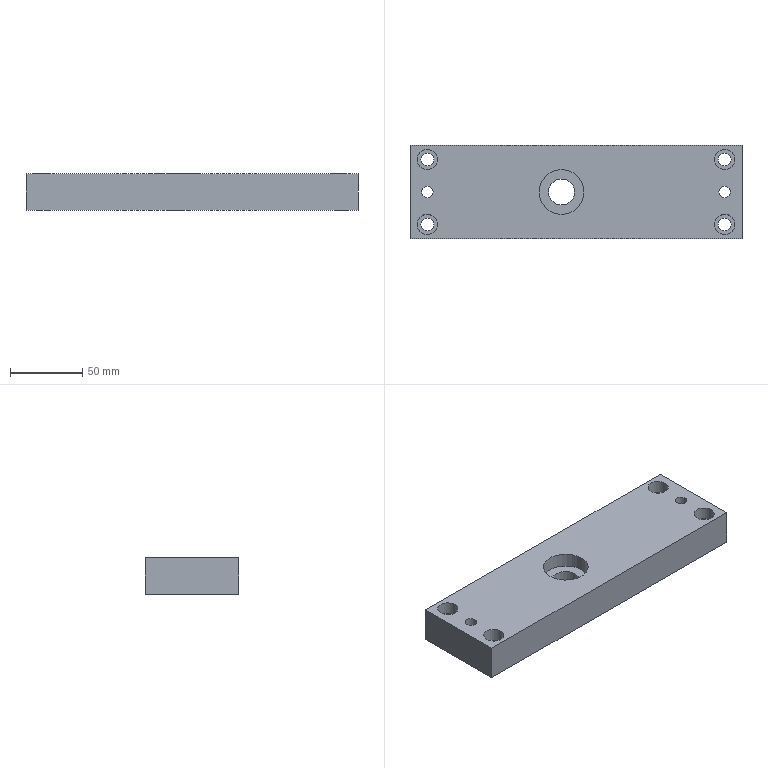Part | STEP file | HYDRAULIC-CYLINDER-BASE2_id482_x_t | 1 solid | 23 faces | box 230 x 65 x 25 mm | volume 350259 mm3 | cylinder 12 | plane 11 | commonest cylinder face diameters 9 x4 14 x4 8 x2 18 x1 31 x1
STEP:
#1=CARTESIAN_POINT('',(90.,-72.5,291.));
#2=VERTEX_POINT('',#1);
#3=CARTESIAN_POINT('',(83.,-72.5,291.));
#4=DIRECTION('',(0.,0.,1.));
#5=DIRECTION('',(1.,0.,0.));
#6=AXIS2_PLACEMENT_3D('',#3,#4,#5);
#7=CIRCLE('',#6,7.);
#8=EDGE_CURVE('',#2,#2,#7,.T.);
#9=ORIENTED_EDGE('',*,*,#8,.F.);
#10=EDGE_LOOP('',(#9));
#11=FACE_BOUND('',#10,.T.);
#12=CARTESIAN_POINT('',(90.,-72.5,300.));
#13=VERTEX_POINT('',#12);
#14=CARTESIAN_POINT('',(83.,-72.5,300.));
#15=DIRECTION('',(0.,0.,-1.));
#16=DIRECTION('',(1.,0.,0.));
#17=AXIS2_PLACEMENT_3D('',#14,#15,#16);
#18=CIRCLE('',#17,7.);
#19=EDGE_CURVE('',#13,#13,#18,.T.);
#20=ORIENTED_EDGE('',*,*,#19,.F.);
#21=EDGE_LOOP('',(#20));
#22=FACE_BOUND('',#21,.T.);
#23=CARTESIAN_POINT('',(83.,-72.5,300.));
#24=DIRECTION('',(0.,0.,1.));
#25=DIRECTION('',(1.,0.,0.));
#26=AXIS2_PLACEMENT_3D('',#23,#24,#25);
#27=CYLINDRICAL_SURFACE('',#26,7.);
#28=ADVANCED_FACE('',(#11,#22),#27,.F.);
#29=CARTESIAN_POINT('',(90.,-27.5,291.));
#30=VERTEX_POINT('',#29);
#31=CARTESIAN_POINT('',(83.,-27.5,291.));
#32=DIRECTION('',(0.,0.,1.));
#33=DIRECTION('',(1.,0.,0.));
#34=AXIS2_PLACEMENT_3D('',#31,#32,#33);
#35=CIRCLE('',#34,7.);
#36=EDGE_CURVE('',#30,#30,#35,.T.);
#37=ORIENTED_EDGE('',*,*,#36,.F.);
#38=EDGE_LOOP('',(#37));
#39=FACE_BOUND('',#38,.T.);
#40=CARTESIAN_POINT('',(90.,-27.5,300.));
#41=VERTEX_POINT('',#40);
#42=CARTESIAN_POINT('',(83.,-27.5,300.));
#43=DIRECTION('',(0.,0.,-1.));
#44=DIRECTION('',(1.,0.,0.));
#45=AXIS2_PLACEMENT_3D('',#42,#43,#44);
#46=CIRCLE('',#45,7.);
#47=EDGE_CURVE('',#41,#41,#46,.T.);
#48=ORIENTED_EDGE('',*,*,#47,.F.);
#49=EDGE_LOOP('',(#48));
#50=FACE_BOUND('',#49,.T.);
#51=CARTESIAN_POINT('',(83.,-27.5,300.));
#52=DIRECTION('',(0.,0.,1.));
#53=DIRECTION('',(1.,0.,0.));
#54=AXIS2_PLACEMENT_3D('',#51,#52,#53);
#55=CYLINDRICAL_SURFACE('',#54,7.);
#56=ADVANCED_FACE('',(#39,#50),#55,.F.);
#57=CARTESIAN_POINT('',(-116.,-27.5,291.));
#58=VERTEX_POINT('',#57);
#59=CARTESIAN_POINT('',(-123.,-27.5,291.));
#60=DIRECTION('',(0.,0.,1.));
#61=DIRECTION('',(1.,0.,0.));
#62=AXIS2_PLACEMENT_3D('',#59,#60,#61);
#63=CIRCLE('',#62,7.);
#64=EDGE_CURVE('',#58,#58,#63,.T.);
#65=ORIENTED_EDGE('',*,*,#64,.F.);
#66=EDGE_LOOP('',(#65));
#67=FACE_BOUND('',#66,.T.);
#68=CARTESIAN_POINT('',(-116.,-27.5,300.));
#69=VERTEX_POINT('',#68);
#70=CARTESIAN_POINT('',(-123.,-27.5,300.));
#71=DIRECTION('',(0.,0.,-1.));
#72=DIRECTION('',(1.,0.,0.));
#73=AXIS2_PLACEMENT_3D('',#70,#71,#72);
#74=CIRCLE('',#73,7.);
#75=EDGE_CURVE('',#69,#69,#74,.T.);
#76=ORIENTED_EDGE('',*,*,#75,.F.);
#77=EDGE_LOOP('',(#76));
#78=FACE_BOUND('',#77,.T.);
#79=CARTESIAN_POINT('',(-123.,-27.5,300.));
#80=DIRECTION('',(0.,0.,1.));
#81=DIRECTION('',(1.,0.,0.));
#82=AXIS2_PLACEMENT_3D('',#79,#80,#81);
#83=CYLINDRICAL_SURFACE('',#82,7.);
#84=ADVANCED_FACE('',(#67,#78),#83,.F.);
#85=CARTESIAN_POINT('',(-116.,-72.5,291.));
#86=VERTEX_POINT('',#85);
#87=CARTESIAN_POINT('',(-123.,-72.5,291.));
#88=DIRECTION('',(0.,0.,1.));
#89=DIRECTION('',(1.,0.,0.));
#90=AXIS2_PLACEMENT_3D('',#87,#88,#89);
#91=CIRCLE('',#90,7.);
#92=EDGE_CURVE('',#86,#86,#91,.T.);
#93=ORIENTED_EDGE('',*,*,#92,.F.);
#94=EDGE_LOOP('',(#93));
#95=FACE_BOUND('',#94,.T.);
#96=CARTESIAN_POINT('',(-116.,-72.5,300.));
#97=VERTEX_POINT('',#96);
#98=CARTESIAN_POINT('',(-123.,-72.5,300.));
#99=DIRECTION('',(0.,0.,-1.));
#100=DIRECTION('',(1.,0.,0.));
#101=AXIS2_PLACEMENT_3D('',#98,#99,#100);
#102=CIRCLE('',#101,7.);
#103=EDGE_CURVE('',#97,#97,#102,.T.);
#104=ORIENTED_EDGE('',*,*,#103,.F.);
#105=EDGE_LOOP('',(#104));
#106=FACE_BOUND('',#105,.T.);
#107=CARTESIAN_POINT('',(-123.,-72.5,300.));
#108=DIRECTION('',(0.,0.,1.));
#109=DIRECTION('',(1.,0.,0.));
#110=AXIS2_PLACEMENT_3D('',#107,#108,#109);
#111=CYLINDRICAL_SURFACE('',#110,7.);
#112=ADVANCED_FACE('',(#95,#106),#111,.F.);
#113=CARTESIAN_POINT('',(-14.5,-50.,290.));
#114=VERTEX_POINT('',#113);
#115=CARTESIAN_POINT('',(-30.,-50.,290.));
#116=DIRECTION('',(0.,0.,1.));
#117=DIRECTION('',(1.,0.,0.));
#118=AXIS2_PLACEMENT_3D('',#115,#116,#117);
#119=CIRCLE('',#118,15.5);
#120=EDGE_CURVE('',#114,#114,#119,.T.);
#121=ORIENTED_EDGE('',*,*,#120,.F.);
#122=EDGE_LOOP('',(#121));
#123=FACE_BOUND('',#122,.T.);
#124=CARTESIAN_POINT('',(-14.5,-50.,300.));
#125=VERTEX_POINT('',#124);
#126=CARTESIAN_POINT('',(-30.,-50.,300.));
#127=DIRECTION('',(0.,0.,-1.));
#128=DIRECTION('',(1.,0.,0.));
#129=AXIS2_PLACEMENT_3D('',#126,#127,#128);
#130=CIRCLE('',#129,15.5);
#131=EDGE_CURVE('',#125,#125,#130,.T.);
#132=ORIENTED_EDGE('',*,*,#131,.F.);
#133=EDGE_LOOP('',(#132));
#134=FACE_BOUND('',#133,.T.);
#135=CARTESIAN_POINT('',(-30.,-50.,300.));
#136=DIRECTION('',(0.,0.,1.));
#137=DIRECTION('',(1.,0.,0.));
#138=AXIS2_PLACEMENT_3D('',#135,#136,#137);
#139=CYLINDRICAL_SURFACE('',#138,15.5);
#140=ADVANCED_FACE('',(#123,#134),#139,.F.);
#141=CARTESIAN_POINT('',(87.5,-27.5,291.));
#142=VERTEX_POINT('',#141);
#143=CARTESIAN_POINT('',(83.,-27.5,291.));
#144=DIRECTION('',(0.,0.,-1.));
#145=DIRECTION('',(1.,0.,0.));
#146=AXIS2_PLACEMENT_3D('',#143,#144,#145);
#147=CIRCLE('',#146,4.5);
#148=EDGE_CURVE('',#142,#142,#147,.T.);
#149=ORIENTED_EDGE('',*,*,#148,.T.);
#150=EDGE_LOOP('',(#149));
#151=FACE_BOUND('',#150,.T.);
#152=ORIENTED_EDGE('',*,*,#36,.T.);
#153=EDGE_LOOP('',(#152));
#154=FACE_BOUND('',#153,.T.);
#155=CARTESIAN_POINT('',(50.126,-0.5,291.));
#156=DIRECTION('',(0.,0.,1.));
#157=DIRECTION('',(1.,0.,0.));
#158=AXIS2_PLACEMENT_3D('',#155,#156,#157);
#159=PLANE('',#158);
#160=ADVANCED_FACE('',(#151,#154),#159,.T.);
#161=CARTESIAN_POINT('',(87.5,-72.5,291.));
#162=VERTEX_POINT('',#161);
#163=CARTESIAN_POINT('',(83.,-72.5,291.));
#164=DIRECTION('',(0.,0.,-1.));
#165=DIRECTION('',(1.,0.,0.));
#166=AXIS2_PLACEMENT_3D('',#163,#164,#165);
#167=CIRCLE('',#166,4.5);
#168=EDGE_CURVE('',#162,#162,#167,.T.);
#169=ORIENTED_EDGE('',*,*,#168,.T.);
#170=EDGE_LOOP('',(#169));
#171=FACE_BOUND('',#170,.T.);
#172=ORIENTED_EDGE('',*,*,#8,.T.);
#173=EDGE_LOOP('',(#172));
#174=FACE_BOUND('',#173,.T.);
#175=CARTESIAN_POINT('',(50.126,-0.5,291.));
#176=DIRECTION('',(0.,0.,1.));
#177=DIRECTION('',(1.,0.,0.));
#178=AXIS2_PLACEMENT_3D('',#175,#176,#177);
#179=PLANE('',#178);
#180=ADVANCED_FACE('',(#171,#174),#179,.T.);
#181=CARTESIAN_POINT('',(-118.5,-27.5,291.));
#182=VERTEX_POINT('',#181);
#183=CARTESIAN_POINT('',(-123.,-27.5,291.));
#184=DIRECTION('',(0.,0.,-1.));
#185=DIRECTION('',(1.,0.,0.));
#186=AXIS2_PLACEMENT_3D('',#183,#184,#185);
#187=CIRCLE('',#186,4.5);
#188=EDGE_CURVE('',#182,#182,#187,.T.);
#189=ORIENTED_EDGE('',*,*,#188,.T.);
#190=EDGE_LOOP('',(#189));
#191=FACE_BOUND('',#190,.T.);
#192=ORIENTED_EDGE('',*,*,#64,.T.);
#193=EDGE_LOOP('',(#192));
#194=FACE_BOUND('',#193,.T.);
#195=CARTESIAN_POINT('',(50.126,-0.5,291.));
#196=DIRECTION('',(0.,0.,1.));
#197=DIRECTION('',(1.,0.,0.));
#198=AXIS2_PLACEMENT_3D('',#195,#196,#197);
#199=PLANE('',#198);
#200=ADVANCED_FACE('',(#191,#194),#199,.T.);
#201=ORIENTED_EDGE('',*,*,#131,.T.);
#202=EDGE_LOOP('',(#201));
#203=FACE_BOUND('',#202,.T.);
#204=ORIENTED_EDGE('',*,*,#75,.T.);
#205=EDGE_LOOP('',(#204));
#206=FACE_BOUND('',#205,.T.);
#207=ORIENTED_EDGE('',*,*,#103,.T.);
#208=EDGE_LOOP('',(#207));
#209=FACE_BOUND('',#208,.T.);
#210=ORIENTED_EDGE('',*,*,#47,.T.);
#211=EDGE_LOOP('',(#210));
#212=FACE_BOUND('',#211,.T.);
#213=ORIENTED_EDGE('',*,*,#19,.T.);
#214=EDGE_LOOP('',(#213));
#215=FACE_BOUND('',#214,.T.);
#216=CARTESIAN_POINT('',(-119.,-50.,300.));
#217=VERTEX_POINT('',#216);
#218=CARTESIAN_POINT('',(-123.,-50.,300.));
#219=DIRECTION('',(0.,0.,-1.));
#220=DIRECTION('',(1.,0.,0.));
#221=AXIS2_PLACEMENT_3D('',#218,#219,#220);
#222=CIRCLE('',#221,4.);
#223=EDGE_CURVE('',#217,#217,#222,.T.);
#224=ORIENTED_EDGE('',*,*,#223,.T.);
#225=EDGE_LOOP('',(#224));
#226=FACE_BOUND('',#225,.T.);
#227=CARTESIAN_POINT('',(87.,-50.,300.));
#228=VERTEX_POINT('',#227);
#229=CARTESIAN_POINT('',(83.,-50.,300.));
#230=DIRECTION('',(0.,0.,-1.));
#231=DIRECTION('',(1.,0.,0.));
#232=AXIS2_PLACEMENT_3D('',#229,#230,#231);
#233=CIRCLE('',#232,4.);
#234=EDGE_CURVE('',#228,#228,#233,.T.);
#235=ORIENTED_EDGE('',*,*,#234,.T.);
#236=EDGE_LOOP('',(#235));
#237=FACE_BOUND('',#236,.T.);
#238=CARTESIAN_POINT('',(95.,-17.5,300.));
#239=VERTEX_POINT('',#238);
#240=CARTESIAN_POINT('',(95.,-82.5,300.));
#241=VERTEX_POINT('',#240);
#242=CARTESIAN_POINT('',(95.,-82.5,300.));
#243=DIRECTION('',(0.,-1.,0.));
#244=VECTOR('',#243,1.);
#245=LINE('',#242,#244);
#246=EDGE_CURVE('',#239,#241,#245,.T.);
#247=ORIENTED_EDGE('',*,*,#246,.F.);
#248=CARTESIAN_POINT('',(-135.,-17.5,300.));
#249=VERTEX_POINT('',#248);
#250=CARTESIAN_POINT('',(95.,-17.5,300.));
#251=DIRECTION('',(1.,0.,0.));
#252=VECTOR('',#251,1.);
#253=LINE('',#250,#252);
#254=EDGE_CURVE('',#249,#239,#253,.T.);
#255=ORIENTED_EDGE('',*,*,#254,.F.);
#256=CARTESIAN_POINT('',(-135.,-82.5,300.));
#257=VERTEX_POINT('',#256);
#258=CARTESIAN_POINT('',(-135.,-17.5,300.));
#259=DIRECTION('',(0.,1.,0.));
#260=VECTOR('',#259,1.);
#261=LINE('',#258,#260);
#262=EDGE_CURVE('',#257,#249,#261,.T.);
#263=ORIENTED_EDGE('',*,*,#262,.F.);
#264=CARTESIAN_POINT('',(-135.,-82.5,300.));
#265=DIRECTION('',(-1.,0.,0.));
#266=VECTOR('',#265,1.);
#267=LINE('',#264,#266);
#268=EDGE_CURVE('',#241,#257,#267,.T.);
#269=ORIENTED_EDGE('',*,*,#268,.F.);
#270=EDGE_LOOP('',(#247,#255,#263,#269));
#271=FACE_BOUND('',#270,.T.);
#272=CARTESIAN_POINT('',(50.126,-0.5,300.));
#273=DIRECTION('',(0.,0.,1.));
#274=DIRECTION('',(1.,0.,0.));
#275=AXIS2_PLACEMENT_3D('',#272,#273,#274);
#276=PLANE('',#275);
#277=ADVANCED_FACE('',(#203,#206,#209,#212,#215,#226,#237,#271),#276,.T.);
#278=CARTESIAN_POINT('',(-118.5,-72.5,291.));
#279=VERTEX_POINT('',#278);
#280=CARTESIAN_POINT('',(-123.,-72.5,291.));
#281=DIRECTION('',(0.,0.,-1.));
#282=DIRECTION('',(1.,0.,0.));
#283=AXIS2_PLACEMENT_3D('',#280,#281,#282);
#284=CIRCLE('',#283,4.5);
#285=EDGE_CURVE('',#279,#279,#284,.T.);
#286=ORIENTED_EDGE('',*,*,#285,.T.);
#287=EDGE_LOOP('',(#286));
#288=FACE_BOUND('',#287,.T.);
#289=ORIENTED_EDGE('',*,*,#92,.T.);
#290=EDGE_LOOP('',(#289));
#291=FACE_BOUND('',#290,.T.);
#292=CARTESIAN_POINT('',(50.126,-0.5,291.));
#293=DIRECTION('',(0.,0.,1.));
#294=DIRECTION('',(1.,0.,0.));
#295=AXIS2_PLACEMENT_3D('',#292,#293,#294);
#296=PLANE('',#295);
#297=ADVANCED_FACE('',(#288,#291),#296,.T.);
#298=CARTESIAN_POINT('',(-21.,-50.,290.));
#299=VERTEX_POINT('',#298);
#300=CARTESIAN_POINT('',(-30.,-50.,290.));
#301=DIRECTION('',(0.,0.,-1.));
#302=DIRECTION('',(1.,0.,0.));
#303=AXIS2_PLACEMENT_3D('',#300,#301,#302);
#304=CIRCLE('',#303,9.);
#305=EDGE_CURVE('',#299,#299,#304,.T.);
#306=ORIENTED_EDGE('',*,*,#305,.T.);
#307=EDGE_LOOP('',(#306));
#308=FACE_BOUND('',#307,.T.);
#309=ORIENTED_EDGE('',*,*,#120,.T.);
#310=EDGE_LOOP('',(#309));
#311=FACE_BOUND('',#310,.T.);
#312=CARTESIAN_POINT('',(50.126,-0.5,290.));
#313=DIRECTION('',(0.,0.,1.));
#314=DIRECTION('',(1.,0.,0.));
#315=AXIS2_PLACEMENT_3D('',#312,#313,#314);
#316=PLANE('',#315);
#317=ADVANCED_FACE('',(#308,#311),#316,.T.);
#318=CARTESIAN_POINT('',(95.,-17.5,275.));
#319=VERTEX_POINT('',#318);
#320=CARTESIAN_POINT('',(95.,-17.5,275.));
#321=DIRECTION('',(0.,0.,1.));
#322=VECTOR('',#321,1.);
#323=LINE('',#320,#322);
#324=EDGE_CURVE('',#319,#239,#323,.T.);
#325=ORIENTED_EDGE('',*,*,#324,.F.);
#326=CARTESIAN_POINT('',(-135.,-17.5,275.));
#327=VERTEX_POINT('',#326);
#328=CARTESIAN_POINT('',(50.126,-17.5,275.));
#329=DIRECTION('',(-1.,0.,0.));
#330=VECTOR('',#329,1.);
#331=LINE('',#328,#330);
#332=EDGE_CURVE('',#319,#327,#331,.T.);
#333=ORIENTED_EDGE('',*,*,#332,.T.);
#334=CARTESIAN_POINT('',(-135.,-17.5,275.));
#335=DIRECTION('',(0.,0.,-1.));
#336=VECTOR('',#335,1.);
#337=LINE('',#334,#336);
#338=EDGE_CURVE('',#249,#327,#337,.T.);
#339=ORIENTED_EDGE('',*,*,#338,.F.);
#340=ORIENTED_EDGE('',*,*,#254,.T.);
#341=EDGE_LOOP('',(#325,#333,#339,#340));
#342=FACE_OUTER_BOUND('',#341,.T.);
#343=CARTESIAN_POINT('',(95.,-17.5,275.));
#344=DIRECTION('',(0.,1.,0.));
#345=DIRECTION('',(0.,0.,1.));
#346=AXIS2_PLACEMENT_3D('',#343,#344,#345);
#347=PLANE('',#346);
#348=ADVANCED_FACE('',(#342),#347,.T.);
#349=ORIENTED_EDGE('',*,*,#338,.T.);
#350=CARTESIAN_POINT('',(-135.,-82.5,275.));
#351=VERTEX_POINT('',#350);
#352=CARTESIAN_POINT('',(-135.,-0.5,275.));
#353=DIRECTION('',(0.,-1.,0.));
#354=VECTOR('',#353,1.);
#355=LINE('',#352,#354);
#356=EDGE_CURVE('',#327,#351,#355,.T.);
#357=ORIENTED_EDGE('',*,*,#356,.T.);
#358=CARTESIAN_POINT('',(-135.,-82.5,275.));
#359=DIRECTION('',(0.,0.,-1.));
#360=VECTOR('',#359,1.);
#361=LINE('',#358,#360);
#362=EDGE_CURVE('',#257,#351,#361,.T.);
#363=ORIENTED_EDGE('',*,*,#362,.F.);
#364=ORIENTED_EDGE('',*,*,#262,.T.);
#365=EDGE_LOOP('',(#349,#357,#363,#364));
#366=FACE_OUTER_BOUND('',#365,.T.);
#367=CARTESIAN_POINT('',(-135.,-17.5,275.));
#368=DIRECTION('',(-1.,0.,0.));
#369=DIRECTION('',(0.,0.,1.));
#370=AXIS2_PLACEMENT_3D('',#367,#368,#369);
#371=PLANE('',#370);
#372=ADVANCED_FACE('',(#366),#371,.T.);
#373=ORIENTED_EDGE('',*,*,#362,.T.);
#374=CARTESIAN_POINT('',(95.,-82.5,275.));
#375=VERTEX_POINT('',#374);
#376=CARTESIAN_POINT('',(50.126,-82.5,275.));
#377=DIRECTION('',(1.,0.,0.));
#378=VECTOR('',#377,1.);
#379=LINE('',#376,#378);
#380=EDGE_CURVE('',#351,#375,#379,.T.);
#381=ORIENTED_EDGE('',*,*,#380,.T.);
#382=CARTESIAN_POINT('',(95.,-82.5,275.));
#383=DIRECTION('',(0.,0.,-1.));
#384=VECTOR('',#383,1.);
#385=LINE('',#382,#384);
#386=EDGE_CURVE('',#241,#375,#385,.T.);
#387=ORIENTED_EDGE('',*,*,#386,.F.);
#388=ORIENTED_EDGE('',*,*,#268,.T.);
#389=EDGE_LOOP('',(#373,#381,#387,#388));
#390=FACE_OUTER_BOUND('',#389,.T.);
#391=CARTESIAN_POINT('',(-135.,-82.5,275.));
#392=DIRECTION('',(0.,-1.,0.));
#393=DIRECTION('',(0.,0.,-1.));
#394=AXIS2_PLACEMENT_3D('',#391,#392,#393);
#395=PLANE('',#394);
#396=ADVANCED_FACE('',(#390),#395,.T.);
#397=ORIENTED_EDGE('',*,*,#386,.T.);
#398=CARTESIAN_POINT('',(95.,-0.5,275.));
#399=DIRECTION('',(0.,1.,0.));
#400=VECTOR('',#399,1.);
#401=LINE('',#398,#400);
#402=EDGE_CURVE('',#375,#319,#401,.T.);
#403=ORIENTED_EDGE('',*,*,#402,.T.);
#404=ORIENTED_EDGE('',*,*,#324,.T.);
#405=ORIENTED_EDGE('',*,*,#246,.T.);
#406=EDGE_LOOP('',(#397,#403,#404,#405));
#407=FACE_OUTER_BOUND('',#406,.T.);
#408=CARTESIAN_POINT('',(95.,-82.5,275.));
#409=DIRECTION('',(1.,0.,0.));
#410=DIRECTION('',(0.,0.,-1.));
#411=AXIS2_PLACEMENT_3D('',#408,#409,#410);
#412=PLANE('',#411);
#413=ADVANCED_FACE('',(#407),#412,.T.);
#414=CARTESIAN_POINT('',(87.5,-27.5,275.));
#415=VERTEX_POINT('',#414);
#416=CARTESIAN_POINT('',(83.,-27.5,275.));
#417=DIRECTION('',(0.,0.,-1.));
#418=DIRECTION('',(1.,0.,0.));
#419=AXIS2_PLACEMENT_3D('',#416,#417,#418);
#420=CIRCLE('',#419,4.5);
#421=EDGE_CURVE('',#415,#415,#420,.T.);
#422=ORIENTED_EDGE('',*,*,#421,.T.);
#423=EDGE_LOOP('',(#422));
#424=FACE_BOUND('',#423,.T.);
#425=ORIENTED_EDGE('',*,*,#148,.F.);
#426=EDGE_LOOP('',(#425));
#427=FACE_BOUND('',#426,.T.);
#428=CARTESIAN_POINT('',(83.,-27.5,275.));
#429=DIRECTION('',(0.,0.,1.));
#430=DIRECTION('',(1.,0.,0.));
#431=AXIS2_PLACEMENT_3D('',#428,#429,#430);
#432=CYLINDRICAL_SURFACE('',#431,4.5);
#433=ADVANCED_FACE('',(#424,#427),#432,.F.);
#434=ORIENTED_EDGE('',*,*,#234,.F.);
#435=EDGE_LOOP('',(#434));
#436=FACE_BOUND('',#435,.T.);
#437=CARTESIAN_POINT('',(87.,-50.,275.));
#438=VERTEX_POINT('',#437);
#439=CARTESIAN_POINT('',(83.,-50.,275.));
#440=DIRECTION('',(0.,0.,-1.));
#441=DIRECTION('',(1.,0.,0.));
#442=AXIS2_PLACEMENT_3D('',#439,#440,#441);
#443=CIRCLE('',#442,4.);
#444=EDGE_CURVE('',#438,#438,#443,.T.);
#445=ORIENTED_EDGE('',*,*,#444,.T.);
#446=EDGE_LOOP('',(#445));
#447=FACE_BOUND('',#446,.T.);
#448=CARTESIAN_POINT('',(83.,-50.,275.));
#449=DIRECTION('',(0.,0.,1.));
#450=DIRECTION('',(1.,0.,0.));
#451=AXIS2_PLACEMENT_3D('',#448,#449,#450);
#452=CYLINDRICAL_SURFACE('',#451,4.);
#453=ADVANCED_FACE('',(#436,#447),#452,.F.);
#454=CARTESIAN_POINT('',(87.5,-72.5,275.));
#455=VERTEX_POINT('',#454);
#456=CARTESIAN_POINT('',(83.,-72.5,275.));
#457=DIRECTION('',(0.,0.,-1.));
#458=DIRECTION('',(1.,0.,0.));
#459=AXIS2_PLACEMENT_3D('',#456,#457,#458);
#460=CIRCLE('',#459,4.5);
#461=EDGE_CURVE('',#455,#455,#460,.T.);
#462=ORIENTED_EDGE('',*,*,#461,.T.);
#463=EDGE_LOOP('',(#462));
#464=FACE_BOUND('',#463,.T.);
#465=ORIENTED_EDGE('',*,*,#168,.F.);
#466=EDGE_LOOP('',(#465));
#467=FACE_BOUND('',#466,.T.);
#468=CARTESIAN_POINT('',(83.,-72.5,275.));
#469=DIRECTION('',(0.,0.,1.));
#470=DIRECTION('',(1.,0.,0.));
#471=AXIS2_PLACEMENT_3D('',#468,#469,#470);
#472=CYLINDRICAL_SURFACE('',#471,4.5);
#473=ADVANCED_FACE('',(#464,#467),#472,.F.);
#474=CARTESIAN_POINT('',(-118.5,-27.5,275.));
#475=VERTEX_POINT('',#474);
#476=CARTESIAN_POINT('',(-123.,-27.5,275.));
#477=DIRECTION('',(0.,0.,-1.));
#478=DIRECTION('',(1.,0.,0.));
#479=AXIS2_PLACEMENT_3D('',#476,#477,#478);
#480=CIRCLE('',#479,4.5);
#481=EDGE_CURVE('',#475,#475,#480,.T.);
#482=ORIENTED_EDGE('',*,*,#481,.T.);
#483=EDGE_LOOP('',(#482));
#484=FACE_BOUND('',#483,.T.);
#485=ORIENTED_EDGE('',*,*,#188,.F.);
#486=EDGE_LOOP('',(#485));
#487=FACE_BOUND('',#486,.T.);
#488=CARTESIAN_POINT('',(-123.,-27.5,275.));
#489=DIRECTION('',(0.,0.,1.));
#490=DIRECTION('',(1.,0.,0.));
#491=AXIS2_PLACEMENT_3D('',#488,#489,#490);
#492=CYLINDRICAL_SURFACE('',#491,4.5);
#493=ADVANCED_FACE('',(#484,#487),#492,.F.);
#494=ORIENTED_EDGE('',*,*,#223,.F.);
#495=EDGE_LOOP('',(#494));
#496=FACE_BOUND('',#495,.T.);
#497=CARTESIAN_POINT('',(-119.,-50.,275.));
#498=VERTEX_POINT('',#497);
#499=CARTESIAN_POINT('',(-123.,-50.,275.));
#500=DIRECTION('',(0.,0.,-1.));
#501=DIRECTION('',(1.,0.,0.));
#502=AXIS2_PLACEMENT_3D('',#499,#500,#501);
#503=CIRCLE('',#502,4.);
#504=EDGE_CURVE('',#498,#498,#503,.T.);
#505=ORIENTED_EDGE('',*,*,#504,.T.);
#506=EDGE_LOOP('',(#505));
#507=FACE_BOUND('',#506,.T.);
#508=CARTESIAN_POINT('',(-123.,-50.,275.));
#509=DIRECTION('',(0.,0.,1.));
#510=DIRECTION('',(1.,0.,0.));
#511=AXIS2_PLACEMENT_3D('',#508,#509,#510);
#512=CYLINDRICAL_SURFACE('',#511,4.);
#513=ADVANCED_FACE('',(#496,#507),#512,.F.);
#514=CARTESIAN_POINT('',(-118.5,-72.5,275.));
#515=VERTEX_POINT('',#514);
#516=CARTESIAN_POINT('',(-123.,-72.5,275.));
#517=DIRECTION('',(0.,0.,-1.));
#518=DIRECTION('',(1.,0.,0.));
#519=AXIS2_PLACEMENT_3D('',#516,#517,#518);
#520=CIRCLE('',#519,4.5);
#521=EDGE_CURVE('',#515,#515,#520,.T.);
#522=ORIENTED_EDGE('',*,*,#521,.T.);
#523=EDGE_LOOP('',(#522));
#524=FACE_BOUND('',#523,.T.);
#525=ORIENTED_EDGE('',*,*,#285,.F.);
#526=EDGE_LOOP('',(#525));
#527=FACE_BOUND('',#526,.T.);
#528=CARTESIAN_POINT('',(-123.,-72.5,275.));
#529=DIRECTION('',(0.,0.,1.));
#530=DIRECTION('',(1.,0.,0.));
#531=AXIS2_PLACEMENT_3D('',#528,#529,#530);
#532=CYLINDRICAL_SURFACE('',#531,4.5);
#533=ADVANCED_FACE('',(#524,#527),#532,.F.);
#534=CARTESIAN_POINT('',(-21.,-50.,275.));
#535=VERTEX_POINT('',#534);
#536=CARTESIAN_POINT('',(-30.,-50.,275.));
#537=DIRECTION('',(0.,0.,-1.));
#538=DIRECTION('',(1.,0.,0.));
#539=AXIS2_PLACEMENT_3D('',#536,#537,#538);
#540=CIRCLE('',#539,9.);
#541=EDGE_CURVE('',#535,#535,#540,.T.);
#542=ORIENTED_EDGE('',*,*,#541,.T.);
#543=EDGE_LOOP('',(#542));
#544=FACE_BOUND('',#543,.T.);
#545=ORIENTED_EDGE('',*,*,#305,.F.);
#546=EDGE_LOOP('',(#545));
#547=FACE_BOUND('',#546,.T.);
#548=CARTESIAN_POINT('',(-30.,-50.,275.));
#549=DIRECTION('',(0.,0.,1.));
#550=DIRECTION('',(1.,0.,0.));
#551=AXIS2_PLACEMENT_3D('',#548,#549,#550);
#552=CYLINDRICAL_SURFACE('',#551,9.);
#553=ADVANCED_FACE('',(#544,#547),#552,.F.);
#554=ORIENTED_EDGE('',*,*,#541,.F.);
#555=EDGE_LOOP('',(#554));
#556=FACE_BOUND('',#555,.T.);
#557=ORIENTED_EDGE('',*,*,#521,.F.);
#558=EDGE_LOOP('',(#557));
#559=FACE_BOUND('',#558,.T.);
#560=ORIENTED_EDGE('',*,*,#504,.F.);
#561=EDGE_LOOP('',(#560));
#562=FACE_BOUND('',#561,.T.);
#563=ORIENTED_EDGE('',*,*,#481,.F.);
#564=EDGE_LOOP('',(#563));
#565=FACE_BOUND('',#564,.T.);
#566=ORIENTED_EDGE('',*,*,#461,.F.);
#567=EDGE_LOOP('',(#566));
#568=FACE_BOUND('',#567,.T.);
#569=ORIENTED_EDGE('',*,*,#444,.F.);
#570=EDGE_LOOP('',(#569));
#571=FACE_BOUND('',#570,.T.);
#572=ORIENTED_EDGE('',*,*,#421,.F.);
#573=EDGE_LOOP('',(#572));
#574=FACE_BOUND('',#573,.T.);
#575=ORIENTED_EDGE('',*,*,#380,.F.);
#576=ORIENTED_EDGE('',*,*,#356,.F.);
#577=ORIENTED_EDGE('',*,*,#332,.F.);
#578=ORIENTED_EDGE('',*,*,#402,.F.);
#579=EDGE_LOOP('',(#575,#576,#577,#578));
#580=FACE_BOUND('',#579,.T.);
#581=CARTESIAN_POINT('',(50.126,-0.5,275.));
#582=DIRECTION('',(0.,0.,1.));
#583=DIRECTION('',(1.,0.,0.));
#584=AXIS2_PLACEMENT_3D('',#581,#582,#583);
#585=PLANE('',#584);
#586=ADVANCED_FACE('',(#556,#559,#562,#565,#568,#571,#574,#580),#585,.F.);
#587=CLOSED_SHELL('',(#28,#56,#84,#112,#140,#160,#180,#200,#277,#297,#317,#348,#372,#396,#413,#433,#453,#473,#493,#513,#533,#553,#586));
#588=MANIFOLD_SOLID_BREP('',#587);
#589=(LENGTH_UNIT()NAMED_UNIT(*)SI_UNIT(.MILLI.,.METRE.));
#590=UNCERTAINTY_MEASURE_WITH_UNIT(LENGTH_MEASURE(0.00002),#589,'','');
#591=(NAMED_UNIT(*)PLANE_ANGLE_UNIT()SI_UNIT($,.RADIAN.));
#592=PLANE_ANGLE_MEASURE_WITH_UNIT(PLANE_ANGLE_MEASURE(0.01745),#591);
#593=DIMENSIONAL_EXPONENTS(0.,0.,0.,0.,0.,0.,0.);
#594=(CONVERSION_BASED_UNIT('DEGREE',#592)NAMED_UNIT(#593)PLANE_ANGLE_UNIT());
#595=(NAMED_UNIT(*)SI_UNIT($,.STERADIAN.)SOLID_ANGLE_UNIT());
#596=(GEOMETRIC_REPRESENTATION_CONTEXT(3)GLOBAL_UNCERTAINTY_ASSIGNED_CONTEXT((#590))GLOBAL_UNIT_ASSIGNED_CONTEXT((#589,#594,#595))REPRESENTATION_CONTEXT('',''));
#597=ADVANCED_BREP_SHAPE_REPRESENTATION('',(#588),#596);